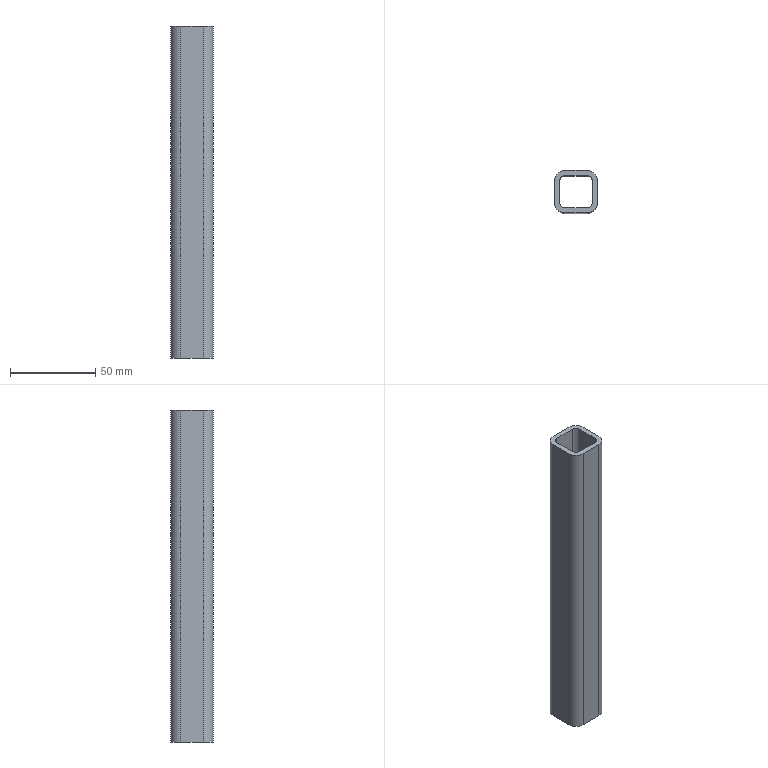Part | STEP file | ISO 10799-2 25x25x3 1784906821110 | 1 solid | 18 faces | box 25 x 25 x 195.176 mm | volume 47003 mm3 | plane 10 | cylinder 8 | commonest cylinder face diameters 6 x4 12 x4
STEP:
#1=CARTESIAN_POINT('',(-6.5,-9.5,195.176));
#2=VERTEX_POINT('',#1);
#3=CARTESIAN_POINT('',(6.5,-9.5,195.176));
#4=VERTEX_POINT('',#3);
#5=CARTESIAN_POINT('',(3.25,-9.5,195.176));
#6=DIRECTION('',(1.,0.,0.));
#7=VECTOR('',#6,10.);
#8=LINE('',#5,#7);
#9=EDGE_CURVE('',#2,#4,#8,.T.);
#10=ORIENTED_EDGE('',*,*,#9,.T.);
#11=CARTESIAN_POINT('',(6.5,-9.5,0.));
#12=VERTEX_POINT('',#11);
#13=CARTESIAN_POINT('',(6.5,-9.5,0.));
#14=DIRECTION('',(0.,0.,1.));
#15=VECTOR('',#14,10.);
#16=LINE('',#13,#15);
#17=EDGE_CURVE('',#12,#4,#16,.T.);
#18=ORIENTED_EDGE('',*,*,#17,.F.);
#19=CARTESIAN_POINT('',(-6.5,-9.5,0.));
#20=VERTEX_POINT('',#19);
#21=CARTESIAN_POINT('',(3.25,-9.5,0.));
#22=DIRECTION('',(1.,0.,0.));
#23=VECTOR('',#22,10.);
#24=LINE('',#21,#23);
#25=EDGE_CURVE('',#20,#12,#24,.T.);
#26=ORIENTED_EDGE('',*,*,#25,.F.);
#27=CARTESIAN_POINT('',(-6.5,-9.5,0.));
#28=DIRECTION('',(0.,0.,1.));
#29=VECTOR('',#28,10.);
#30=LINE('',#27,#29);
#31=EDGE_CURVE('',#20,#2,#30,.T.);
#32=ORIENTED_EDGE('',*,*,#31,.T.);
#33=EDGE_LOOP('',(#10,#18,#26,#32));
#34=FACE_OUTER_BOUND('',#33,.T.);
#35=CARTESIAN_POINT('',(6.5,-9.5,0.));
#36=DIRECTION('',(0.,-1.,0.));
#37=DIRECTION('',(0.,0.,-1.));
#38=AXIS2_PLACEMENT_3D('',#35,#36,#37);
#39=PLANE('',#38);
#40=ADVANCED_FACE('',(#34),#39,.F.);
#41=CARTESIAN_POINT('',(9.5,-6.5,195.176));
#42=VERTEX_POINT('',#41);
#43=CARTESIAN_POINT('',(6.5,-6.5,195.176));
#44=DIRECTION('',(0.,0.,1.));
#45=DIRECTION('',(0.,1.,0.));
#46=AXIS2_PLACEMENT_3D('',#43,#44,#45);
#47=CIRCLE('',#46,3.);
#48=EDGE_CURVE('',#4,#42,#47,.T.);
#49=ORIENTED_EDGE('',*,*,#48,.T.);
#50=CARTESIAN_POINT('',(9.5,-6.5,0.));
#51=VERTEX_POINT('',#50);
#52=CARTESIAN_POINT('',(9.5,-6.5,0.));
#53=DIRECTION('',(0.,0.,1.));
#54=VECTOR('',#53,10.);
#55=LINE('',#52,#54);
#56=EDGE_CURVE('',#51,#42,#55,.T.);
#57=ORIENTED_EDGE('',*,*,#56,.F.);
#58=CARTESIAN_POINT('',(6.5,-6.5,0.));
#59=DIRECTION('',(0.,0.,1.));
#60=DIRECTION('',(0.,1.,0.));
#61=AXIS2_PLACEMENT_3D('',#58,#59,#60);
#62=CIRCLE('',#61,3.);
#63=EDGE_CURVE('',#12,#51,#62,.T.);
#64=ORIENTED_EDGE('',*,*,#63,.F.);
#65=ORIENTED_EDGE('',*,*,#17,.T.);
#66=EDGE_LOOP('',(#49,#57,#64,#65));
#67=FACE_OUTER_BOUND('',#66,.T.);
#68=CARTESIAN_POINT('',(6.5,-6.5,0.));
#69=DIRECTION('',(0.,0.,1.));
#70=DIRECTION('',(0.,1.,0.));
#71=AXIS2_PLACEMENT_3D('',#68,#69,#70);
#72=CYLINDRICAL_SURFACE('',#71,3.);
#73=ADVANCED_FACE('',(#67),#72,.F.);
#74=CARTESIAN_POINT('',(9.5,6.5,195.176));
#75=VERTEX_POINT('',#74);
#76=CARTESIAN_POINT('',(9.5,3.25,195.176));
#77=DIRECTION('',(0.,1.,0.));
#78=VECTOR('',#77,10.);
#79=LINE('',#76,#78);
#80=EDGE_CURVE('',#42,#75,#79,.T.);
#81=ORIENTED_EDGE('',*,*,#80,.T.);
#82=CARTESIAN_POINT('',(9.5,6.5,0.));
#83=VERTEX_POINT('',#82);
#84=CARTESIAN_POINT('',(9.5,6.5,0.));
#85=DIRECTION('',(0.,0.,1.));
#86=VECTOR('',#85,10.);
#87=LINE('',#84,#86);
#88=EDGE_CURVE('',#83,#75,#87,.T.);
#89=ORIENTED_EDGE('',*,*,#88,.F.);
#90=CARTESIAN_POINT('',(9.5,3.25,0.));
#91=DIRECTION('',(0.,1.,0.));
#92=VECTOR('',#91,10.);
#93=LINE('',#90,#92);
#94=EDGE_CURVE('',#51,#83,#93,.T.);
#95=ORIENTED_EDGE('',*,*,#94,.F.);
#96=ORIENTED_EDGE('',*,*,#56,.T.);
#97=EDGE_LOOP('',(#81,#89,#95,#96));
#98=FACE_OUTER_BOUND('',#97,.T.);
#99=CARTESIAN_POINT('',(9.5,6.5,0.));
#100=DIRECTION('',(1.,0.,0.));
#101=DIRECTION('',(0.,0.,-1.));
#102=AXIS2_PLACEMENT_3D('',#99,#100,#101);
#103=PLANE('',#102);
#104=ADVANCED_FACE('',(#98),#103,.F.);
#105=CARTESIAN_POINT('',(6.5,9.5,195.176));
#106=VERTEX_POINT('',#105);
#107=CARTESIAN_POINT('',(6.5,6.5,195.176));
#108=DIRECTION('',(0.,0.,1.));
#109=DIRECTION('',(-1.,0.,0.));
#110=AXIS2_PLACEMENT_3D('',#107,#108,#109);
#111=CIRCLE('',#110,3.);
#112=EDGE_CURVE('',#75,#106,#111,.T.);
#113=ORIENTED_EDGE('',*,*,#112,.T.);
#114=CARTESIAN_POINT('',(6.5,9.5,0.));
#115=VERTEX_POINT('',#114);
#116=CARTESIAN_POINT('',(6.5,9.5,0.));
#117=DIRECTION('',(0.,0.,1.));
#118=VECTOR('',#117,10.);
#119=LINE('',#116,#118);
#120=EDGE_CURVE('',#115,#106,#119,.T.);
#121=ORIENTED_EDGE('',*,*,#120,.F.);
#122=CARTESIAN_POINT('',(6.5,6.5,0.));
#123=DIRECTION('',(0.,0.,1.));
#124=DIRECTION('',(-1.,0.,0.));
#125=AXIS2_PLACEMENT_3D('',#122,#123,#124);
#126=CIRCLE('',#125,3.);
#127=EDGE_CURVE('',#83,#115,#126,.T.);
#128=ORIENTED_EDGE('',*,*,#127,.F.);
#129=ORIENTED_EDGE('',*,*,#88,.T.);
#130=EDGE_LOOP('',(#113,#121,#128,#129));
#131=FACE_OUTER_BOUND('',#130,.T.);
#132=CARTESIAN_POINT('',(6.5,6.5,0.));
#133=DIRECTION('',(0.,0.,1.));
#134=DIRECTION('',(-1.,0.,0.));
#135=AXIS2_PLACEMENT_3D('',#132,#133,#134);
#136=CYLINDRICAL_SURFACE('',#135,3.);
#137=ADVANCED_FACE('',(#131),#136,.F.);
#138=CARTESIAN_POINT('',(12.5,6.5,195.176));
#139=VERTEX_POINT('',#138);
#140=CARTESIAN_POINT('',(12.5,-6.5,195.176));
#141=VERTEX_POINT('',#140);
#142=CARTESIAN_POINT('',(12.5,3.25,195.176));
#143=DIRECTION('',(0.,-1.,0.));
#144=VECTOR('',#143,10.);
#145=LINE('',#142,#144);
#146=EDGE_CURVE('',#139,#141,#145,.T.);
#147=ORIENTED_EDGE('',*,*,#146,.T.);
#148=CARTESIAN_POINT('',(12.5,-6.5,0.));
#149=VERTEX_POINT('',#148);
#150=CARTESIAN_POINT('',(12.5,-6.5,0.));
#151=DIRECTION('',(0.,0.,1.));
#152=VECTOR('',#151,10.);
#153=LINE('',#150,#152);
#154=EDGE_CURVE('',#149,#141,#153,.T.);
#155=ORIENTED_EDGE('',*,*,#154,.F.);
#156=CARTESIAN_POINT('',(12.5,6.5,0.));
#157=VERTEX_POINT('',#156);
#158=CARTESIAN_POINT('',(12.5,3.25,0.));
#159=DIRECTION('',(0.,-1.,0.));
#160=VECTOR('',#159,10.);
#161=LINE('',#158,#160);
#162=EDGE_CURVE('',#157,#149,#161,.T.);
#163=ORIENTED_EDGE('',*,*,#162,.F.);
#164=CARTESIAN_POINT('',(12.5,6.5,0.));
#165=DIRECTION('',(0.,0.,1.));
#166=VECTOR('',#165,10.);
#167=LINE('',#164,#166);
#168=EDGE_CURVE('',#157,#139,#167,.T.);
#169=ORIENTED_EDGE('',*,*,#168,.T.);
#170=EDGE_LOOP('',(#147,#155,#163,#169));
#171=FACE_OUTER_BOUND('',#170,.T.);
#172=CARTESIAN_POINT('',(12.5,6.5,0.));
#173=DIRECTION('',(1.,0.,0.));
#174=DIRECTION('',(0.,0.,-1.));
#175=AXIS2_PLACEMENT_3D('',#172,#173,#174);
#176=PLANE('',#175);
#177=ADVANCED_FACE('',(#171),#176,.T.);
#178=CARTESIAN_POINT('',(6.5,-12.5,195.176));
#179=VERTEX_POINT('',#178);
#180=CARTESIAN_POINT('',(6.5,-6.5,195.176));
#181=DIRECTION('',(0.,0.,-1.));
#182=DIRECTION('',(0.,1.,0.));
#183=AXIS2_PLACEMENT_3D('',#180,#181,#182);
#184=CIRCLE('',#183,6.);
#185=EDGE_CURVE('',#141,#179,#184,.T.);
#186=ORIENTED_EDGE('',*,*,#185,.T.);
#187=CARTESIAN_POINT('',(6.5,-12.5,0.));
#188=VERTEX_POINT('',#187);
#189=CARTESIAN_POINT('',(6.5,-12.5,0.));
#190=DIRECTION('',(0.,0.,1.));
#191=VECTOR('',#190,10.);
#192=LINE('',#189,#191);
#193=EDGE_CURVE('',#188,#179,#192,.T.);
#194=ORIENTED_EDGE('',*,*,#193,.F.);
#195=CARTESIAN_POINT('',(6.5,-6.5,0.));
#196=DIRECTION('',(0.,0.,-1.));
#197=DIRECTION('',(0.,1.,0.));
#198=AXIS2_PLACEMENT_3D('',#195,#196,#197);
#199=CIRCLE('',#198,6.);
#200=EDGE_CURVE('',#149,#188,#199,.T.);
#201=ORIENTED_EDGE('',*,*,#200,.F.);
#202=ORIENTED_EDGE('',*,*,#154,.T.);
#203=EDGE_LOOP('',(#186,#194,#201,#202));
#204=FACE_OUTER_BOUND('',#203,.T.);
#205=CARTESIAN_POINT('',(6.5,-6.5,0.));
#206=DIRECTION('',(0.,0.,1.));
#207=DIRECTION('',(0.,1.,0.));
#208=AXIS2_PLACEMENT_3D('',#205,#206,#207);
#209=CYLINDRICAL_SURFACE('',#208,6.);
#210=ADVANCED_FACE('',(#204),#209,.T.);
#211=CARTESIAN_POINT('',(-6.5,-12.5,195.176));
#212=VERTEX_POINT('',#211);
#213=CARTESIAN_POINT('',(3.25,-12.5,195.176));
#214=DIRECTION('',(-1.,0.,0.));
#215=VECTOR('',#214,10.);
#216=LINE('',#213,#215);
#217=EDGE_CURVE('',#179,#212,#216,.T.);
#218=ORIENTED_EDGE('',*,*,#217,.T.);
#219=CARTESIAN_POINT('',(-6.5,-12.5,0.));
#220=VERTEX_POINT('',#219);
#221=CARTESIAN_POINT('',(-6.5,-12.5,0.));
#222=DIRECTION('',(0.,0.,1.));
#223=VECTOR('',#222,10.);
#224=LINE('',#221,#223);
#225=EDGE_CURVE('',#220,#212,#224,.T.);
#226=ORIENTED_EDGE('',*,*,#225,.F.);
#227=CARTESIAN_POINT('',(3.25,-12.5,0.));
#228=DIRECTION('',(-1.,0.,0.));
#229=VECTOR('',#228,10.);
#230=LINE('',#227,#229);
#231=EDGE_CURVE('',#188,#220,#230,.T.);
#232=ORIENTED_EDGE('',*,*,#231,.F.);
#233=ORIENTED_EDGE('',*,*,#193,.T.);
#234=EDGE_LOOP('',(#218,#226,#232,#233));
#235=FACE_OUTER_BOUND('',#234,.T.);
#236=CARTESIAN_POINT('',(6.5,-12.5,0.));
#237=DIRECTION('',(0.,-1.,0.));
#238=DIRECTION('',(0.,0.,-1.));
#239=AXIS2_PLACEMENT_3D('',#236,#237,#238);
#240=PLANE('',#239);
#241=ADVANCED_FACE('',(#235),#240,.T.);
#242=CARTESIAN_POINT('',(-12.5,-6.5,195.176));
#243=VERTEX_POINT('',#242);
#244=CARTESIAN_POINT('',(-6.5,-6.5,195.176));
#245=DIRECTION('',(0.,0.,-1.));
#246=DIRECTION('',(1.,0.,0.));
#247=AXIS2_PLACEMENT_3D('',#244,#245,#246);
#248=CIRCLE('',#247,6.);
#249=EDGE_CURVE('',#212,#243,#248,.T.);
#250=ORIENTED_EDGE('',*,*,#249,.T.);
#251=CARTESIAN_POINT('',(-12.5,-6.5,0.));
#252=VERTEX_POINT('',#251);
#253=CARTESIAN_POINT('',(-12.5,-6.5,0.));
#254=DIRECTION('',(0.,0.,1.));
#255=VECTOR('',#254,10.);
#256=LINE('',#253,#255);
#257=EDGE_CURVE('',#252,#243,#256,.T.);
#258=ORIENTED_EDGE('',*,*,#257,.F.);
#259=CARTESIAN_POINT('',(-6.5,-6.5,0.));
#260=DIRECTION('',(0.,0.,-1.));
#261=DIRECTION('',(1.,0.,0.));
#262=AXIS2_PLACEMENT_3D('',#259,#260,#261);
#263=CIRCLE('',#262,6.);
#264=EDGE_CURVE('',#220,#252,#263,.T.);
#265=ORIENTED_EDGE('',*,*,#264,.F.);
#266=ORIENTED_EDGE('',*,*,#225,.T.);
#267=EDGE_LOOP('',(#250,#258,#265,#266));
#268=FACE_OUTER_BOUND('',#267,.T.);
#269=CARTESIAN_POINT('',(-6.5,-6.5,0.));
#270=DIRECTION('',(0.,0.,1.));
#271=DIRECTION('',(1.,0.,0.));
#272=AXIS2_PLACEMENT_3D('',#269,#270,#271);
#273=CYLINDRICAL_SURFACE('',#272,6.);
#274=ADVANCED_FACE('',(#268),#273,.T.);
#275=CARTESIAN_POINT('',(-6.5,9.5,195.176));
#276=VERTEX_POINT('',#275);
#277=CARTESIAN_POINT('',(-3.25,9.5,195.176));
#278=DIRECTION('',(-1.,0.,0.));
#279=VECTOR('',#278,10.);
#280=LINE('',#277,#279);
#281=EDGE_CURVE('',#106,#276,#280,.T.);
#282=ORIENTED_EDGE('',*,*,#281,.T.);
#283=CARTESIAN_POINT('',(-6.5,9.5,0.));
#284=VERTEX_POINT('',#283);
#285=CARTESIAN_POINT('',(-6.5,9.5,0.));
#286=DIRECTION('',(0.,0.,1.));
#287=VECTOR('',#286,10.);
#288=LINE('',#285,#287);
#289=EDGE_CURVE('',#284,#276,#288,.T.);
#290=ORIENTED_EDGE('',*,*,#289,.F.);
#291=CARTESIAN_POINT('',(-3.25,9.5,0.));
#292=DIRECTION('',(-1.,0.,0.));
#293=VECTOR('',#292,10.);
#294=LINE('',#291,#293);
#295=EDGE_CURVE('',#115,#284,#294,.T.);
#296=ORIENTED_EDGE('',*,*,#295,.F.);
#297=ORIENTED_EDGE('',*,*,#120,.T.);
#298=EDGE_LOOP('',(#282,#290,#296,#297));
#299=FACE_OUTER_BOUND('',#298,.T.);
#300=CARTESIAN_POINT('',(-6.5,9.5,0.));
#301=DIRECTION('',(0.,1.,0.));
#302=DIRECTION('',(0.,0.,1.));
#303=AXIS2_PLACEMENT_3D('',#300,#301,#302);
#304=PLANE('',#303);
#305=ADVANCED_FACE('',(#299),#304,.F.);
#306=CARTESIAN_POINT('',(-9.5,-6.5,195.176));
#307=VERTEX_POINT('',#306);
#308=CARTESIAN_POINT('',(-6.5,-6.5,195.176));
#309=DIRECTION('',(0.,0.,1.));
#310=DIRECTION('',(1.,0.,0.));
#311=AXIS2_PLACEMENT_3D('',#308,#309,#310);
#312=CIRCLE('',#311,3.);
#313=EDGE_CURVE('',#307,#2,#312,.T.);
#314=ORIENTED_EDGE('',*,*,#313,.T.);
#315=ORIENTED_EDGE('',*,*,#31,.F.);
#316=CARTESIAN_POINT('',(-9.5,-6.5,0.));
#317=VERTEX_POINT('',#316);
#318=CARTESIAN_POINT('',(-6.5,-6.5,0.));
#319=DIRECTION('',(0.,0.,1.));
#320=DIRECTION('',(1.,0.,0.));
#321=AXIS2_PLACEMENT_3D('',#318,#319,#320);
#322=CIRCLE('',#321,3.);
#323=EDGE_CURVE('',#317,#20,#322,.T.);
#324=ORIENTED_EDGE('',*,*,#323,.F.);
#325=CARTESIAN_POINT('',(-9.5,-6.5,0.));
#326=DIRECTION('',(0.,0.,1.));
#327=VECTOR('',#326,10.);
#328=LINE('',#325,#327);
#329=EDGE_CURVE('',#317,#307,#328,.T.);
#330=ORIENTED_EDGE('',*,*,#329,.T.);
#331=EDGE_LOOP('',(#314,#315,#324,#330));
#332=FACE_OUTER_BOUND('',#331,.T.);
#333=CARTESIAN_POINT('',(-6.5,-6.5,0.));
#334=DIRECTION('',(0.,0.,1.));
#335=DIRECTION('',(1.,0.,0.));
#336=AXIS2_PLACEMENT_3D('',#333,#334,#335);
#337=CYLINDRICAL_SURFACE('',#336,3.);
#338=ADVANCED_FACE('',(#332),#337,.F.);
#339=CARTESIAN_POINT('',(-9.5,6.5,195.176));
#340=VERTEX_POINT('',#339);
#341=CARTESIAN_POINT('',(-9.5,-3.25,195.176));
#342=DIRECTION('',(0.,-1.,0.));
#343=VECTOR('',#342,10.);
#344=LINE('',#341,#343);
#345=EDGE_CURVE('',#340,#307,#344,.T.);
#346=ORIENTED_EDGE('',*,*,#345,.T.);
#347=ORIENTED_EDGE('',*,*,#329,.F.);
#348=CARTESIAN_POINT('',(-9.5,6.5,0.));
#349=VERTEX_POINT('',#348);
#350=CARTESIAN_POINT('',(-9.5,-3.25,0.));
#351=DIRECTION('',(0.,-1.,0.));
#352=VECTOR('',#351,10.);
#353=LINE('',#350,#352);
#354=EDGE_CURVE('',#349,#317,#353,.T.);
#355=ORIENTED_EDGE('',*,*,#354,.F.);
#356=CARTESIAN_POINT('',(-9.5,6.5,0.));
#357=DIRECTION('',(0.,0.,1.));
#358=VECTOR('',#357,10.);
#359=LINE('',#356,#358);
#360=EDGE_CURVE('',#349,#340,#359,.T.);
#361=ORIENTED_EDGE('',*,*,#360,.T.);
#362=EDGE_LOOP('',(#346,#347,#355,#361));
#363=FACE_OUTER_BOUND('',#362,.T.);
#364=CARTESIAN_POINT('',(-9.5,-6.5,0.));
#365=DIRECTION('',(-1.,0.,0.));
#366=DIRECTION('',(0.,0.,1.));
#367=AXIS2_PLACEMENT_3D('',#364,#365,#366);
#368=PLANE('',#367);
#369=ADVANCED_FACE('',(#363),#368,.F.);
#370=CARTESIAN_POINT('',(-6.5,6.5,195.176));
#371=DIRECTION('',(0.,0.,1.));
#372=DIRECTION('',(0.,-1.,0.));
#373=AXIS2_PLACEMENT_3D('',#370,#371,#372);
#374=CIRCLE('',#373,3.);
#375=EDGE_CURVE('',#276,#340,#374,.T.);
#376=ORIENTED_EDGE('',*,*,#375,.T.);
#377=ORIENTED_EDGE('',*,*,#360,.F.);
#378=CARTESIAN_POINT('',(-6.5,6.5,0.));
#379=DIRECTION('',(0.,0.,1.));
#380=DIRECTION('',(0.,-1.,0.));
#381=AXIS2_PLACEMENT_3D('',#378,#379,#380);
#382=CIRCLE('',#381,3.);
#383=EDGE_CURVE('',#284,#349,#382,.T.);
#384=ORIENTED_EDGE('',*,*,#383,.F.);
#385=ORIENTED_EDGE('',*,*,#289,.T.);
#386=EDGE_LOOP('',(#376,#377,#384,#385));
#387=FACE_OUTER_BOUND('',#386,.T.);
#388=CARTESIAN_POINT('',(-6.5,6.5,0.));
#389=DIRECTION('',(0.,0.,1.));
#390=DIRECTION('',(0.,-1.,0.));
#391=AXIS2_PLACEMENT_3D('',#388,#389,#390);
#392=CYLINDRICAL_SURFACE('',#391,3.);
#393=ADVANCED_FACE('',(#387),#392,.F.);
#394=CARTESIAN_POINT('',(-12.5,6.5,195.176));
#395=VERTEX_POINT('',#394);
#396=CARTESIAN_POINT('',(-12.5,-3.25,195.176));
#397=DIRECTION('',(0.,1.,0.));
#398=VECTOR('',#397,10.);
#399=LINE('',#396,#398);
#400=EDGE_CURVE('',#243,#395,#399,.T.);
#401=ORIENTED_EDGE('',*,*,#400,.T.);
#402=CARTESIAN_POINT('',(-12.5,6.5,0.));
#403=VERTEX_POINT('',#402);
#404=CARTESIAN_POINT('',(-12.5,6.5,0.));
#405=DIRECTION('',(0.,0.,1.));
#406=VECTOR('',#405,10.);
#407=LINE('',#404,#406);
#408=EDGE_CURVE('',#403,#395,#407,.T.);
#409=ORIENTED_EDGE('',*,*,#408,.F.);
#410=CARTESIAN_POINT('',(-12.5,-3.25,0.));
#411=DIRECTION('',(0.,1.,0.));
#412=VECTOR('',#411,10.);
#413=LINE('',#410,#412);
#414=EDGE_CURVE('',#252,#403,#413,.T.);
#415=ORIENTED_EDGE('',*,*,#414,.F.);
#416=ORIENTED_EDGE('',*,*,#257,.T.);
#417=EDGE_LOOP('',(#401,#409,#415,#416));
#418=FACE_OUTER_BOUND('',#417,.T.);
#419=CARTESIAN_POINT('',(-12.5,-6.5,0.));
#420=DIRECTION('',(-1.,0.,0.));
#421=DIRECTION('',(0.,0.,1.));
#422=AXIS2_PLACEMENT_3D('',#419,#420,#421);
#423=PLANE('',#422);
#424=ADVANCED_FACE('',(#418),#423,.T.);
#425=CARTESIAN_POINT('',(-6.5,12.5,195.176));
#426=VERTEX_POINT('',#425);
#427=CARTESIAN_POINT('',(-6.5,6.5,195.176));
#428=DIRECTION('',(0.,0.,-1.));
#429=DIRECTION('',(0.,-1.,0.));
#430=AXIS2_PLACEMENT_3D('',#427,#428,#429);
#431=CIRCLE('',#430,6.);
#432=EDGE_CURVE('',#395,#426,#431,.T.);
#433=ORIENTED_EDGE('',*,*,#432,.T.);
#434=CARTESIAN_POINT('',(-6.5,12.5,0.));
#435=VERTEX_POINT('',#434);
#436=CARTESIAN_POINT('',(-6.5,12.5,0.));
#437=DIRECTION('',(0.,0.,1.));
#438=VECTOR('',#437,10.);
#439=LINE('',#436,#438);
#440=EDGE_CURVE('',#435,#426,#439,.T.);
#441=ORIENTED_EDGE('',*,*,#440,.F.);
#442=CARTESIAN_POINT('',(-6.5,6.5,0.));
#443=DIRECTION('',(0.,0.,-1.));
#444=DIRECTION('',(0.,-1.,0.));
#445=AXIS2_PLACEMENT_3D('',#442,#443,#444);
#446=CIRCLE('',#445,6.);
#447=EDGE_CURVE('',#403,#435,#446,.T.);
#448=ORIENTED_EDGE('',*,*,#447,.F.);
#449=ORIENTED_EDGE('',*,*,#408,.T.);
#450=EDGE_LOOP('',(#433,#441,#448,#449));
#451=FACE_OUTER_BOUND('',#450,.T.);
#452=CARTESIAN_POINT('',(-6.5,6.5,0.));
#453=DIRECTION('',(0.,0.,1.));
#454=DIRECTION('',(0.,-1.,0.));
#455=AXIS2_PLACEMENT_3D('',#452,#453,#454);
#456=CYLINDRICAL_SURFACE('',#455,6.);
#457=ADVANCED_FACE('',(#451),#456,.T.);
#458=CARTESIAN_POINT('',(6.5,12.5,195.176));
#459=VERTEX_POINT('',#458);
#460=CARTESIAN_POINT('',(-3.25,12.5,195.176));
#461=DIRECTION('',(1.,0.,0.));
#462=VECTOR('',#461,10.);
#463=LINE('',#460,#462);
#464=EDGE_CURVE('',#426,#459,#463,.T.);
#465=ORIENTED_EDGE('',*,*,#464,.T.);
#466=CARTESIAN_POINT('',(6.5,12.5,0.));
#467=VERTEX_POINT('',#466);
#468=CARTESIAN_POINT('',(6.5,12.5,0.));
#469=DIRECTION('',(0.,0.,1.));
#470=VECTOR('',#469,10.);
#471=LINE('',#468,#470);
#472=EDGE_CURVE('',#467,#459,#471,.T.);
#473=ORIENTED_EDGE('',*,*,#472,.F.);
#474=CARTESIAN_POINT('',(-3.25,12.5,0.));
#475=DIRECTION('',(1.,0.,0.));
#476=VECTOR('',#475,10.);
#477=LINE('',#474,#476);
#478=EDGE_CURVE('',#435,#467,#477,.T.);
#479=ORIENTED_EDGE('',*,*,#478,.F.);
#480=ORIENTED_EDGE('',*,*,#440,.T.);
#481=EDGE_LOOP('',(#465,#473,#479,#480));
#482=FACE_OUTER_BOUND('',#481,.T.);
#483=CARTESIAN_POINT('',(-6.5,12.5,0.));
#484=DIRECTION('',(0.,1.,0.));
#485=DIRECTION('',(0.,0.,1.));
#486=AXIS2_PLACEMENT_3D('',#483,#484,#485);
#487=PLANE('',#486);
#488=ADVANCED_FACE('',(#482),#487,.T.);
#489=CARTESIAN_POINT('',(6.5,6.5,195.176));
#490=DIRECTION('',(0.,0.,-1.));
#491=DIRECTION('',(-1.,0.,0.));
#492=AXIS2_PLACEMENT_3D('',#489,#490,#491);
#493=CIRCLE('',#492,6.);
#494=EDGE_CURVE('',#459,#139,#493,.T.);
#495=ORIENTED_EDGE('',*,*,#494,.T.);
#496=ORIENTED_EDGE('',*,*,#168,.F.);
#497=CARTESIAN_POINT('',(6.5,6.5,0.));
#498=DIRECTION('',(0.,0.,-1.));
#499=DIRECTION('',(-1.,0.,0.));
#500=AXIS2_PLACEMENT_3D('',#497,#498,#499);
#501=CIRCLE('',#500,6.);
#502=EDGE_CURVE('',#467,#157,#501,.T.);
#503=ORIENTED_EDGE('',*,*,#502,.F.);
#504=ORIENTED_EDGE('',*,*,#472,.T.);
#505=EDGE_LOOP('',(#495,#496,#503,#504));
#506=FACE_OUTER_BOUND('',#505,.T.);
#507=CARTESIAN_POINT('',(6.5,6.5,0.));
#508=DIRECTION('',(0.,0.,1.));
#509=DIRECTION('',(-1.,0.,0.));
#510=AXIS2_PLACEMENT_3D('',#507,#508,#509);
#511=CYLINDRICAL_SURFACE('',#510,6.);
#512=ADVANCED_FACE('',(#506),#511,.T.);
#513=ORIENTED_EDGE('',*,*,#414,.T.);
#514=ORIENTED_EDGE('',*,*,#447,.T.);
#515=ORIENTED_EDGE('',*,*,#478,.T.);
#516=ORIENTED_EDGE('',*,*,#502,.T.);
#517=ORIENTED_EDGE('',*,*,#162,.T.);
#518=ORIENTED_EDGE('',*,*,#200,.T.);
#519=ORIENTED_EDGE('',*,*,#231,.T.);
#520=ORIENTED_EDGE('',*,*,#264,.T.);
#521=EDGE_LOOP('',(#513,#514,#515,#516,#517,#518,#519,#520));
#522=FACE_OUTER_BOUND('',#521,.T.);
#523=ORIENTED_EDGE('',*,*,#295,.T.);
#524=ORIENTED_EDGE('',*,*,#383,.T.);
#525=ORIENTED_EDGE('',*,*,#354,.T.);
#526=ORIENTED_EDGE('',*,*,#323,.T.);
#527=ORIENTED_EDGE('',*,*,#25,.T.);
#528=ORIENTED_EDGE('',*,*,#63,.T.);
#529=ORIENTED_EDGE('',*,*,#94,.T.);
#530=ORIENTED_EDGE('',*,*,#127,.T.);
#531=EDGE_LOOP('',(#523,#524,#525,#526,#527,#528,#529,#530));
#532=FACE_BOUND('',#531,.T.);
#533=CARTESIAN_POINT('',(0.,0.,0.));
#534=DIRECTION('',(0.,0.,1.));
#535=DIRECTION('',(1.,0.,0.));
#536=AXIS2_PLACEMENT_3D('',#533,#534,#535);
#537=PLANE('',#536);
#538=ADVANCED_FACE('',(#522,#532),#537,.F.);
#539=ORIENTED_EDGE('',*,*,#400,.F.);
#540=ORIENTED_EDGE('',*,*,#249,.F.);
#541=ORIENTED_EDGE('',*,*,#217,.F.);
#542=ORIENTED_EDGE('',*,*,#185,.F.);
#543=ORIENTED_EDGE('',*,*,#146,.F.);
#544=ORIENTED_EDGE('',*,*,#494,.F.);
#545=ORIENTED_EDGE('',*,*,#464,.F.);
#546=ORIENTED_EDGE('',*,*,#432,.F.);
#547=EDGE_LOOP('',(#539,#540,#541,#542,#543,#544,#545,#546));
#548=FACE_OUTER_BOUND('',#547,.T.);
#549=ORIENTED_EDGE('',*,*,#281,.F.);
#550=ORIENTED_EDGE('',*,*,#112,.F.);
#551=ORIENTED_EDGE('',*,*,#80,.F.);
#552=ORIENTED_EDGE('',*,*,#48,.F.);
#553=ORIENTED_EDGE('',*,*,#9,.F.);
#554=ORIENTED_EDGE('',*,*,#313,.F.);
#555=ORIENTED_EDGE('',*,*,#345,.F.);
#556=ORIENTED_EDGE('',*,*,#375,.F.);
#557=EDGE_LOOP('',(#549,#550,#551,#552,#553,#554,#555,#556));
#558=FACE_BOUND('',#557,.T.);
#559=CARTESIAN_POINT('',(0.,0.,195.176));
#560=DIRECTION('',(0.,0.,1.));
#561=DIRECTION('',(1.,0.,0.));
#562=AXIS2_PLACEMENT_3D('',#559,#560,#561);
#563=PLANE('',#562);
#564=ADVANCED_FACE('',(#548,#558),#563,.T.);
#565=CLOSED_SHELL('',(#40,#73,#104,#137,#177,#210,#241,#274,#305,#338,#369,#393,#424,#457,#488,#512,#538,#564));
#566=MANIFOLD_SOLID_BREP('',#565);
#567=(LENGTH_UNIT()NAMED_UNIT(*)SI_UNIT(.MILLI.,.METRE.));
#568=UNCERTAINTY_MEASURE_WITH_UNIT(LENGTH_MEASURE(0.01),#567,'','');
#569=(NAMED_UNIT(*)PLANE_ANGLE_UNIT()SI_UNIT($,.RADIAN.));
#570=(NAMED_UNIT(*)SI_UNIT($,.STERADIAN.)SOLID_ANGLE_UNIT());
#571=(GEOMETRIC_REPRESENTATION_CONTEXT(3)GLOBAL_UNCERTAINTY_ASSIGNED_CONTEXT((#568))GLOBAL_UNIT_ASSIGNED_CONTEXT((#567,#569,#570))REPRESENTATION_CONTEXT('',''));
#572=ADVANCED_BREP_SHAPE_REPRESENTATION('',(#566),#571);